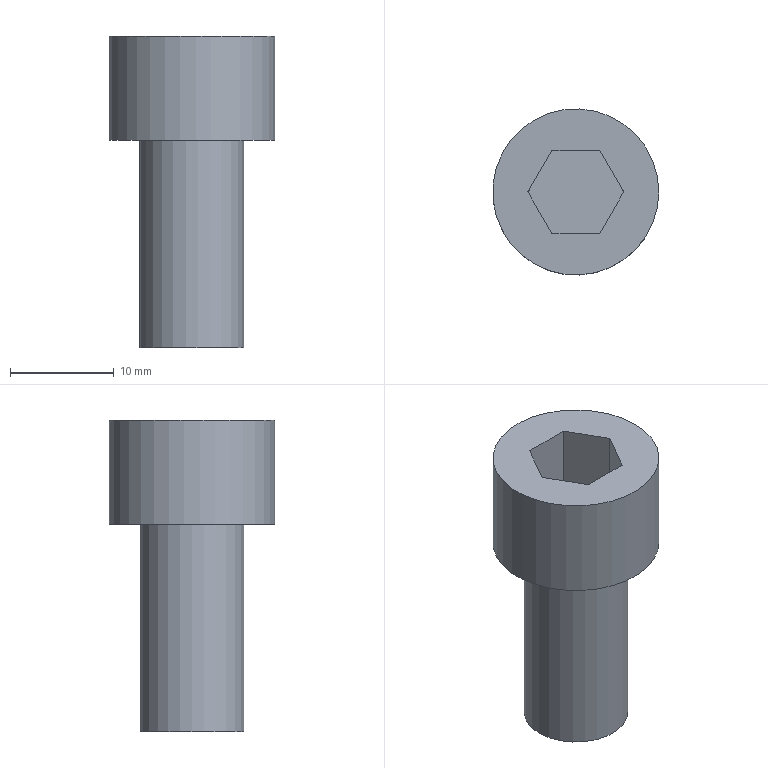Part | STEP file | 冲床-300配套压波_id46_x_t | 1 solid | 12 faces | box 16 x 16 x 30 mm | volume 3216 mm3 | plane 10 | cylinder 2 | commonest cylinder face diameters 10 x1 16 x1
STEP:
#1=CARTESIAN_POINT('',(1208.,-117.5,24.));
#2=VERTEX_POINT('',#1);
#3=CARTESIAN_POINT('',(1200.,-117.5,24.));
#4=DIRECTION('',(0.,0.,1.));
#5=DIRECTION('',(1.,0.,0.));
#6=AXIS2_PLACEMENT_3D('',#3,#4,#5);
#7=CIRCLE('',#6,8.);
#8=EDGE_CURVE('',#2,#2,#7,.T.);
#9=ORIENTED_EDGE('',*,*,#8,.T.);
#10=EDGE_LOOP('',(#9));
#11=FACE_BOUND('',#10,.T.);
#12=CARTESIAN_POINT('',(1197.691,-113.5,24.));
#13=VERTEX_POINT('',#12);
#14=CARTESIAN_POINT('',(1202.309,-113.5,24.));
#15=VERTEX_POINT('',#14);
#16=CARTESIAN_POINT('',(1197.691,-113.5,24.));
#17=DIRECTION('',(1.,0.,0.));
#18=VECTOR('',#17,1.);
#19=LINE('',#16,#18);
#20=EDGE_CURVE('',#13,#15,#19,.T.);
#21=ORIENTED_EDGE('',*,*,#20,.T.);
#22=CARTESIAN_POINT('',(1204.619,-117.5,24.));
#23=VERTEX_POINT('',#22);
#24=CARTESIAN_POINT('',(1202.309,-113.5,24.));
#25=DIRECTION('',(0.5,-0.866,0.));
#26=VECTOR('',#25,1.);
#27=LINE('',#24,#26);
#28=EDGE_CURVE('',#15,#23,#27,.T.);
#29=ORIENTED_EDGE('',*,*,#28,.T.);
#30=CARTESIAN_POINT('',(1202.309,-121.5,24.));
#31=VERTEX_POINT('',#30);
#32=CARTESIAN_POINT('',(1204.619,-117.5,24.));
#33=DIRECTION('',(-0.5,-0.866,0.));
#34=VECTOR('',#33,1.);
#35=LINE('',#32,#34);
#36=EDGE_CURVE('',#23,#31,#35,.T.);
#37=ORIENTED_EDGE('',*,*,#36,.T.);
#38=CARTESIAN_POINT('',(1197.691,-121.5,24.));
#39=VERTEX_POINT('',#38);
#40=CARTESIAN_POINT('',(1202.309,-121.5,24.));
#41=DIRECTION('',(-1.,0.,0.));
#42=VECTOR('',#41,1.);
#43=LINE('',#40,#42);
#44=EDGE_CURVE('',#31,#39,#43,.T.);
#45=ORIENTED_EDGE('',*,*,#44,.T.);
#46=CARTESIAN_POINT('',(1195.381,-117.5,24.));
#47=VERTEX_POINT('',#46);
#48=CARTESIAN_POINT('',(1197.691,-121.5,24.));
#49=DIRECTION('',(-0.5,0.866,0.));
#50=VECTOR('',#49,1.);
#51=LINE('',#48,#50);
#52=EDGE_CURVE('',#39,#47,#51,.T.);
#53=ORIENTED_EDGE('',*,*,#52,.T.);
#54=CARTESIAN_POINT('',(1195.381,-117.5,24.));
#55=DIRECTION('',(0.5,0.866,0.));
#56=VECTOR('',#55,1.);
#57=LINE('',#54,#56);
#58=EDGE_CURVE('',#47,#13,#57,.T.);
#59=ORIENTED_EDGE('',*,*,#58,.T.);
#60=EDGE_LOOP('',(#21,#29,#37,#45,#53,#59));
#61=FACE_BOUND('',#60,.T.);
#62=CARTESIAN_POINT('',(1208.,-117.5,24.));
#63=DIRECTION('',(0.,0.,-1.));
#64=DIRECTION('',(-1.,0.,0.));
#65=AXIS2_PLACEMENT_3D('',#62,#63,#64);
#66=PLANE('',#65);
#67=ADVANCED_FACE('',(#11,#61),#66,.F.);
#68=ORIENTED_EDGE('',*,*,#8,.F.);
#69=EDGE_LOOP('',(#68));
#70=FACE_BOUND('',#69,.T.);
#71=CARTESIAN_POINT('',(1208.,-117.5,14.));
#72=VERTEX_POINT('',#71);
#73=CARTESIAN_POINT('',(1200.,-117.5,14.));
#74=DIRECTION('',(0.,0.,1.));
#75=DIRECTION('',(1.,0.,0.));
#76=AXIS2_PLACEMENT_3D('',#73,#74,#75);
#77=CIRCLE('',#76,8.);
#78=EDGE_CURVE('',#72,#72,#77,.T.);
#79=ORIENTED_EDGE('',*,*,#78,.T.);
#80=EDGE_LOOP('',(#79));
#81=FACE_BOUND('',#80,.T.);
#82=CARTESIAN_POINT('',(1200.,-117.5,15.1));
#83=DIRECTION('',(0.,0.,1.));
#84=DIRECTION('',(1.,0.,0.));
#85=AXIS2_PLACEMENT_3D('',#82,#83,#84);
#86=CYLINDRICAL_SURFACE('',#85,8.);
#87=ADVANCED_FACE('',(#70,#81),#86,.T.);
#88=ORIENTED_EDGE('',*,*,#78,.F.);
#89=EDGE_LOOP('',(#88));
#90=FACE_BOUND('',#89,.T.);
#91=CARTESIAN_POINT('',(1205.,-117.5,14.));
#92=VERTEX_POINT('',#91);
#93=CARTESIAN_POINT('',(1200.,-117.5,14.));
#94=DIRECTION('',(0.,0.,1.));
#95=DIRECTION('',(1.,0.,0.));
#96=AXIS2_PLACEMENT_3D('',#93,#94,#95);
#97=CIRCLE('',#96,5.);
#98=EDGE_CURVE('',#92,#92,#97,.T.);
#99=ORIENTED_EDGE('',*,*,#98,.T.);
#100=EDGE_LOOP('',(#99));
#101=FACE_BOUND('',#100,.T.);
#102=CARTESIAN_POINT('',(1205.,-117.5,14.));
#103=DIRECTION('',(0.,0.,1.));
#104=DIRECTION('',(1.,0.,0.));
#105=AXIS2_PLACEMENT_3D('',#102,#103,#104);
#106=PLANE('',#105);
#107=ADVANCED_FACE('',(#90,#101),#106,.F.);
#108=ORIENTED_EDGE('',*,*,#98,.F.);
#109=EDGE_LOOP('',(#108));
#110=FACE_BOUND('',#109,.T.);
#111=CARTESIAN_POINT('',(1205.,-117.5,-6.));
#112=VERTEX_POINT('',#111);
#113=CARTESIAN_POINT('',(1200.,-117.5,-6.));
#114=DIRECTION('',(0.,0.,1.));
#115=DIRECTION('',(1.,0.,0.));
#116=AXIS2_PLACEMENT_3D('',#113,#114,#115);
#117=CIRCLE('',#116,5.);
#118=EDGE_CURVE('',#112,#112,#117,.T.);
#119=ORIENTED_EDGE('',*,*,#118,.T.);
#120=EDGE_LOOP('',(#119));
#121=FACE_BOUND('',#120,.T.);
#122=CARTESIAN_POINT('',(1200.,-117.5,15.1));
#123=DIRECTION('',(0.,0.,1.));
#124=DIRECTION('',(1.,0.,0.));
#125=AXIS2_PLACEMENT_3D('',#122,#123,#124);
#126=CYLINDRICAL_SURFACE('',#125,5.);
#127=ADVANCED_FACE('',(#110,#121),#126,.T.);
#128=ORIENTED_EDGE('',*,*,#118,.F.);
#129=EDGE_LOOP('',(#128));
#130=FACE_OUTER_BOUND('',#129,.T.);
#131=CARTESIAN_POINT('',(1200.,-117.5,-6.));
#132=DIRECTION('',(0.,0.,1.));
#133=DIRECTION('',(1.,0.,0.));
#134=AXIS2_PLACEMENT_3D('',#131,#132,#133);
#135=PLANE('',#134);
#136=ADVANCED_FACE('',(#130),#135,.F.);
#137=ORIENTED_EDGE('',*,*,#20,.F.);
#138=CARTESIAN_POINT('',(1197.691,-113.5,17.4));
#139=VERTEX_POINT('',#138);
#140=CARTESIAN_POINT('',(1197.691,-113.5,17.4));
#141=DIRECTION('',(0.,0.,-1.));
#142=VECTOR('',#141,1.);
#143=LINE('',#140,#142);
#144=EDGE_CURVE('',#13,#139,#143,.T.);
#145=ORIENTED_EDGE('',*,*,#144,.T.);
#146=CARTESIAN_POINT('',(1202.309,-113.5,17.4));
#147=VERTEX_POINT('',#146);
#148=CARTESIAN_POINT('',(1197.691,-113.5,17.4));
#149=DIRECTION('',(-1.,0.,0.));
#150=VECTOR('',#149,1.);
#151=LINE('',#148,#150);
#152=EDGE_CURVE('',#147,#139,#151,.T.);
#153=ORIENTED_EDGE('',*,*,#152,.F.);
#154=CARTESIAN_POINT('',(1202.309,-113.5,17.4));
#155=DIRECTION('',(0.,0.,-1.));
#156=VECTOR('',#155,1.);
#157=LINE('',#154,#156);
#158=EDGE_CURVE('',#15,#147,#157,.T.);
#159=ORIENTED_EDGE('',*,*,#158,.F.);
#160=EDGE_LOOP('',(#137,#145,#153,#159));
#161=FACE_OUTER_BOUND('',#160,.T.);
#162=CARTESIAN_POINT('',(1197.691,-113.5,17.4));
#163=DIRECTION('',(0.,-1.,0.));
#164=DIRECTION('',(1.,0.,0.));
#165=AXIS2_PLACEMENT_3D('',#162,#163,#164);
#166=PLANE('',#165);
#167=ADVANCED_FACE('',(#161),#166,.T.);
#168=ORIENTED_EDGE('',*,*,#28,.F.);
#169=ORIENTED_EDGE('',*,*,#158,.T.);
#170=CARTESIAN_POINT('',(1204.619,-117.5,17.4));
#171=VERTEX_POINT('',#170);
#172=CARTESIAN_POINT('',(1202.309,-113.5,17.4));
#173=DIRECTION('',(-0.5,0.866,0.));
#174=VECTOR('',#173,1.);
#175=LINE('',#172,#174);
#176=EDGE_CURVE('',#171,#147,#175,.T.);
#177=ORIENTED_EDGE('',*,*,#176,.F.);
#178=CARTESIAN_POINT('',(1204.619,-117.5,17.4));
#179=DIRECTION('',(0.,0.,-1.));
#180=VECTOR('',#179,1.);
#181=LINE('',#178,#180);
#182=EDGE_CURVE('',#23,#171,#181,.T.);
#183=ORIENTED_EDGE('',*,*,#182,.F.);
#184=EDGE_LOOP('',(#168,#169,#177,#183));
#185=FACE_OUTER_BOUND('',#184,.T.);
#186=CARTESIAN_POINT('',(1202.309,-113.5,17.4));
#187=DIRECTION('',(-0.866,-0.5,0.));
#188=DIRECTION('',(0.5,-0.866,0.));
#189=AXIS2_PLACEMENT_3D('',#186,#187,#188);
#190=PLANE('',#189);
#191=ADVANCED_FACE('',(#185),#190,.T.);
#192=ORIENTED_EDGE('',*,*,#36,.F.);
#193=ORIENTED_EDGE('',*,*,#182,.T.);
#194=CARTESIAN_POINT('',(1202.309,-121.5,17.4));
#195=VERTEX_POINT('',#194);
#196=CARTESIAN_POINT('',(1204.619,-117.5,17.4));
#197=DIRECTION('',(0.5,0.866,0.));
#198=VECTOR('',#197,1.);
#199=LINE('',#196,#198);
#200=EDGE_CURVE('',#195,#171,#199,.T.);
#201=ORIENTED_EDGE('',*,*,#200,.F.);
#202=CARTESIAN_POINT('',(1202.309,-121.5,17.4));
#203=DIRECTION('',(0.,0.,-1.));
#204=VECTOR('',#203,1.);
#205=LINE('',#202,#204);
#206=EDGE_CURVE('',#31,#195,#205,.T.);
#207=ORIENTED_EDGE('',*,*,#206,.F.);
#208=EDGE_LOOP('',(#192,#193,#201,#207));
#209=FACE_OUTER_BOUND('',#208,.T.);
#210=CARTESIAN_POINT('',(1204.619,-117.5,17.4));
#211=DIRECTION('',(-0.866,0.5,0.));
#212=DIRECTION('',(-0.5,-0.866,0.));
#213=AXIS2_PLACEMENT_3D('',#210,#211,#212);
#214=PLANE('',#213);
#215=ADVANCED_FACE('',(#209),#214,.T.);
#216=ORIENTED_EDGE('',*,*,#44,.F.);
#217=ORIENTED_EDGE('',*,*,#206,.T.);
#218=CARTESIAN_POINT('',(1197.691,-121.5,17.4));
#219=VERTEX_POINT('',#218);
#220=CARTESIAN_POINT('',(1202.309,-121.5,17.4));
#221=DIRECTION('',(1.,0.,0.));
#222=VECTOR('',#221,1.);
#223=LINE('',#220,#222);
#224=EDGE_CURVE('',#219,#195,#223,.T.);
#225=ORIENTED_EDGE('',*,*,#224,.F.);
#226=CARTESIAN_POINT('',(1197.691,-121.5,17.4));
#227=DIRECTION('',(0.,0.,-1.));
#228=VECTOR('',#227,1.);
#229=LINE('',#226,#228);
#230=EDGE_CURVE('',#39,#219,#229,.T.);
#231=ORIENTED_EDGE('',*,*,#230,.F.);
#232=EDGE_LOOP('',(#216,#217,#225,#231));
#233=FACE_OUTER_BOUND('',#232,.T.);
#234=CARTESIAN_POINT('',(1202.309,-121.5,17.4));
#235=DIRECTION('',(0.,1.,0.));
#236=DIRECTION('',(0.,0.,1.));
#237=AXIS2_PLACEMENT_3D('',#234,#235,#236);
#238=PLANE('',#237);
#239=ADVANCED_FACE('',(#233),#238,.T.);
#240=ORIENTED_EDGE('',*,*,#52,.F.);
#241=ORIENTED_EDGE('',*,*,#230,.T.);
#242=CARTESIAN_POINT('',(1195.381,-117.5,17.4));
#243=VERTEX_POINT('',#242);
#244=CARTESIAN_POINT('',(1197.691,-121.5,17.4));
#245=DIRECTION('',(0.5,-0.866,0.));
#246=VECTOR('',#245,1.);
#247=LINE('',#244,#246);
#248=EDGE_CURVE('',#243,#219,#247,.T.);
#249=ORIENTED_EDGE('',*,*,#248,.F.);
#250=CARTESIAN_POINT('',(1195.381,-117.5,17.4));
#251=DIRECTION('',(0.,0.,-1.));
#252=VECTOR('',#251,1.);
#253=LINE('',#250,#252);
#254=EDGE_CURVE('',#47,#243,#253,.T.);
#255=ORIENTED_EDGE('',*,*,#254,.F.);
#256=EDGE_LOOP('',(#240,#241,#249,#255));
#257=FACE_OUTER_BOUND('',#256,.T.);
#258=CARTESIAN_POINT('',(1197.691,-121.5,17.4));
#259=DIRECTION('',(0.866,0.5,0.));
#260=DIRECTION('',(-0.5,0.866,0.));
#261=AXIS2_PLACEMENT_3D('',#258,#259,#260);
#262=PLANE('',#261);
#263=ADVANCED_FACE('',(#257),#262,.T.);
#264=ORIENTED_EDGE('',*,*,#58,.F.);
#265=ORIENTED_EDGE('',*,*,#254,.T.);
#266=CARTESIAN_POINT('',(1195.381,-117.5,17.4));
#267=DIRECTION('',(-0.5,-0.866,0.));
#268=VECTOR('',#267,1.);
#269=LINE('',#266,#268);
#270=EDGE_CURVE('',#139,#243,#269,.T.);
#271=ORIENTED_EDGE('',*,*,#270,.F.);
#272=ORIENTED_EDGE('',*,*,#144,.F.);
#273=EDGE_LOOP('',(#264,#265,#271,#272));
#274=FACE_OUTER_BOUND('',#273,.T.);
#275=CARTESIAN_POINT('',(1195.381,-117.5,17.4));
#276=DIRECTION('',(0.866,-0.5,0.));
#277=DIRECTION('',(0.5,0.866,0.));
#278=AXIS2_PLACEMENT_3D('',#275,#276,#277);
#279=PLANE('',#278);
#280=ADVANCED_FACE('',(#274),#279,.T.);
#281=ORIENTED_EDGE('',*,*,#152,.T.);
#282=ORIENTED_EDGE('',*,*,#270,.T.);
#283=ORIENTED_EDGE('',*,*,#248,.T.);
#284=ORIENTED_EDGE('',*,*,#224,.T.);
#285=ORIENTED_EDGE('',*,*,#200,.T.);
#286=ORIENTED_EDGE('',*,*,#176,.T.);
#287=EDGE_LOOP('',(#281,#282,#283,#284,#285,#286));
#288=FACE_OUTER_BOUND('',#287,.T.);
#289=CARTESIAN_POINT('',(1200.,-117.5,17.4));
#290=DIRECTION('',(0.,0.,-1.));
#291=DIRECTION('',(-1.,0.,0.));
#292=AXIS2_PLACEMENT_3D('',#289,#290,#291);
#293=PLANE('',#292);
#294=ADVANCED_FACE('',(#288),#293,.F.);
#295=CLOSED_SHELL('',(#67,#87,#107,#127,#136,#167,#191,#215,#239,#263,#280,#294));
#296=MANIFOLD_SOLID_BREP('',#295);
#297=(LENGTH_UNIT()NAMED_UNIT(*)SI_UNIT(.MILLI.,.METRE.));
#298=UNCERTAINTY_MEASURE_WITH_UNIT(LENGTH_MEASURE(0.00002),#297,'','');
#299=(NAMED_UNIT(*)PLANE_ANGLE_UNIT()SI_UNIT($,.RADIAN.));
#300=PLANE_ANGLE_MEASURE_WITH_UNIT(PLANE_ANGLE_MEASURE(0.01745),#299);
#301=DIMENSIONAL_EXPONENTS(0.,0.,0.,0.,0.,0.,0.);
#302=(CONVERSION_BASED_UNIT('DEGREE',#300)NAMED_UNIT(#301)PLANE_ANGLE_UNIT());
#303=(NAMED_UNIT(*)SI_UNIT($,.STERADIAN.)SOLID_ANGLE_UNIT());
#304=(GEOMETRIC_REPRESENTATION_CONTEXT(3)GLOBAL_UNCERTAINTY_ASSIGNED_CONTEXT((#298))GLOBAL_UNIT_ASSIGNED_CONTEXT((#297,#302,#303))REPRESENTATION_CONTEXT('',''));
#305=ADVANCED_BREP_SHAPE_REPRESENTATION('',(#296),#304);